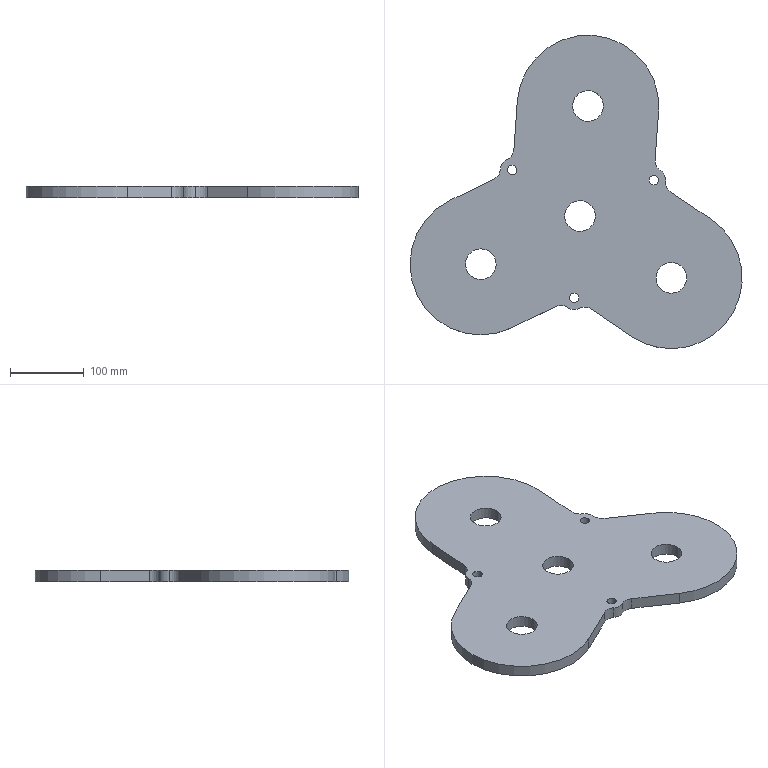Part | SolidWorks | features BaseBody 1 | 1 solid | 37 faces | box 450.446 x 425.125 x 16 mm | volume 1740357 mm3 | cylinder 29 | plane 8 | commonest cylinder face diameters 32 x11 41.6 x8 12.8 x6 192 x4
STEP:
#1=CARTESIAN_POINT('',(-327.08,104.201,479.4));
#2=VERTEX_POINT('',#1);
#3=CARTESIAN_POINT('',(-327.068,104.358,479.4));
#4=VERTEX_POINT('',#3);
#5=CARTESIAN_POINT('',(-311.122,103.052,479.4));
#6=DIRECTION('',(0.,0.,-1.));
#7=DIRECTION('',(-0.9974,0.07181,0.));
#8=AXIS2_PLACEMENT_3D('',#5,#6,#7);
#9=CIRCLE('',#8,16.);
#10=EDGE_CURVE('',#2,#4,#9,.T.);
#11=ORIENTED_EDGE('',*,*,#10,.F.);
#12=CARTESIAN_POINT('',(-327.08,104.201,463.4));
#13=VERTEX_POINT('',#12);
#14=CARTESIAN_POINT('',(-327.08,104.201,524.655));
#15=DIRECTION('',(0.,0.,-1.));
#16=VECTOR('',#15,1000.);
#17=LINE('',#14,#16);
#18=EDGE_CURVE('',#2,#13,#17,.T.);
#19=ORIENTED_EDGE('',*,*,#18,.T.);
#20=CARTESIAN_POINT('',(-327.068,104.358,463.4));
#21=VERTEX_POINT('',#20);
#22=CARTESIAN_POINT('',(-311.122,103.052,463.4));
#23=DIRECTION('',(0.,0.,1.));
#24=DIRECTION('',(-0.9974,0.07181,0.));
#25=AXIS2_PLACEMENT_3D('',#22,#23,#24);
#26=CIRCLE('',#25,16.);
#27=EDGE_CURVE('',#21,#13,#26,.T.);
#28=ORIENTED_EDGE('',*,*,#27,.F.);
#29=CARTESIAN_POINT('',(-327.068,104.358,524.655));
#30=DIRECTION('',(0.,0.,-1.));
#31=VECTOR('',#30,1000.);
#32=LINE('',#29,#31);
#33=EDGE_CURVE('',#4,#21,#32,.T.);
#34=ORIENTED_EDGE('',*,*,#33,.F.);
#35=EDGE_LOOP('',(#11,#19,#28,#34));
#36=FACE_OUTER_BOUND('',#35,.T.);
#37=CARTESIAN_POINT('',(-311.122,103.052,524.655));
#38=DIRECTION('',(0.,0.,-1.));
#39=DIRECTION('',(-0.9974,0.07181,0.));
#40=AXIS2_PLACEMENT_3D('',#37,#38,#39);
#41=CYLINDRICAL_SURFACE('',#40,16.);
#42=ADVANCED_FACE('',(#36),#41,.F.);
#43=CARTESIAN_POINT('',(-541.45,119.952,479.4));
#44=VERTEX_POINT('',#43);
#45=CARTESIAN_POINT('',(-528.683,119.033,479.4));
#46=VERTEX_POINT('',#45);
#47=CARTESIAN_POINT('',(-535.066,119.493,479.4));
#48=DIRECTION('',(0.,0.,1.));
#49=DIRECTION('',(-0.9974,0.07181,0.));
#50=AXIS2_PLACEMENT_3D('',#47,#48,#49);
#51=CIRCLE('',#50,6.4);
#52=EDGE_CURVE('',#44,#46,#51,.T.);
#53=ORIENTED_EDGE('',*,*,#52,.T.);
#54=CARTESIAN_POINT('',(-528.683,119.033,463.4));
#55=VERTEX_POINT('',#54);
#56=CARTESIAN_POINT('',(-528.683,119.033,524.655));
#57=DIRECTION('',(0.,0.,-1.));
#58=VECTOR('',#57,1000.);
#59=LINE('',#56,#58);
#60=EDGE_CURVE('',#46,#55,#59,.T.);
#61=ORIENTED_EDGE('',*,*,#60,.T.);
#62=CARTESIAN_POINT('',(-541.45,119.952,463.4));
#63=VERTEX_POINT('',#62);
#64=CARTESIAN_POINT('',(-535.066,119.493,463.4));
#65=DIRECTION('',(0.,0.,-1.));
#66=DIRECTION('',(-0.9974,0.07181,0.));
#67=AXIS2_PLACEMENT_3D('',#64,#65,#66);
#68=CIRCLE('',#67,6.4);
#69=EDGE_CURVE('',#55,#63,#68,.T.);
#70=ORIENTED_EDGE('',*,*,#69,.T.);
#71=CARTESIAN_POINT('',(-541.45,119.952,524.655));
#72=DIRECTION('',(0.,0.,-1.));
#73=VECTOR('',#72,1000.);
#74=LINE('',#71,#73);
#75=EDGE_CURVE('',#44,#63,#74,.T.);
#76=ORIENTED_EDGE('',*,*,#75,.F.);
#77=EDGE_LOOP('',(#53,#61,#70,#76));
#78=FACE_OUTER_BOUND('',#77,.T.);
#79=CARTESIAN_POINT('',(-535.066,119.493,524.655));
#80=DIRECTION('',(0.,0.,-1.));
#81=DIRECTION('',(-0.9974,0.07181,0.));
#82=AXIS2_PLACEMENT_3D('',#79,#80,#81);
#83=CYLINDRICAL_SURFACE('',#82,6.4);
#84=ADVANCED_FACE('',(#78),#83,.F.);
#85=CARTESIAN_POINT('',(-551.025,120.642,479.4));
#86=VERTEX_POINT('',#85);
#87=CARTESIAN_POINT('',(-551.036,120.484,479.4));
#88=VERTEX_POINT('',#87);
#89=CARTESIAN_POINT('',(-535.066,119.493,479.4));
#90=DIRECTION('',(0.,0.,1.));
#91=DIRECTION('',(-0.9974,0.07181,0.));
#92=AXIS2_PLACEMENT_3D('',#89,#90,#91);
#93=CIRCLE('',#92,16.);
#94=EDGE_CURVE('',#86,#88,#93,.T.);
#95=ORIENTED_EDGE('',*,*,#94,.F.);
#96=CARTESIAN_POINT('',(-551.025,120.642,463.4));
#97=VERTEX_POINT('',#96);
#98=CARTESIAN_POINT('',(-551.025,120.642,524.655));
#99=DIRECTION('',(0.,0.,-1.));
#100=VECTOR('',#99,1000.);
#101=LINE('',#98,#100);
#102=EDGE_CURVE('',#86,#97,#101,.T.);
#103=ORIENTED_EDGE('',*,*,#102,.T.);
#104=CARTESIAN_POINT('',(-551.036,120.484,463.4));
#105=VERTEX_POINT('',#104);
#106=CARTESIAN_POINT('',(-535.066,119.493,463.4));
#107=DIRECTION('',(0.,0.,-1.));
#108=DIRECTION('',(-0.9974,0.07181,0.));
#109=AXIS2_PLACEMENT_3D('',#106,#107,#108);
#110=CIRCLE('',#109,16.);
#111=EDGE_CURVE('',#105,#97,#110,.T.);
#112=ORIENTED_EDGE('',*,*,#111,.F.);
#113=CARTESIAN_POINT('',(-551.036,120.484,524.655));
#114=DIRECTION('',(0.,0.,1.));
#115=VECTOR('',#114,1000.);
#116=LINE('',#113,#115);
#117=EDGE_CURVE('',#105,#88,#116,.T.);
#118=ORIENTED_EDGE('',*,*,#117,.T.);
#119=EDGE_LOOP('',(#95,#103,#112,#118));
#120=FACE_OUTER_BOUND('',#119,.T.);
#121=CARTESIAN_POINT('',(-535.066,119.493,524.655));
#122=DIRECTION('',(0.,0.,-1.));
#123=DIRECTION('',(-0.9974,0.07181,0.));
#124=AXIS2_PLACEMENT_3D('',#121,#122,#123);
#125=CYLINDRICAL_SURFACE('',#124,16.);
#126=ADVANCED_FACE('',(#120),#125,.T.);
#127=CARTESIAN_POINT('',(-349.398,106.125,479.4));
#128=VERTEX_POINT('',#127);
#129=CARTESIAN_POINT('',(-336.631,105.205,479.4));
#130=VERTEX_POINT('',#129);
#131=CARTESIAN_POINT('',(-343.015,105.665,479.4));
#132=DIRECTION('',(0.,0.,1.));
#133=DIRECTION('',(-0.9974,0.07181,0.));
#134=AXIS2_PLACEMENT_3D('',#131,#132,#133);
#135=CIRCLE('',#134,6.4);
#136=EDGE_CURVE('',#128,#130,#135,.T.);
#137=ORIENTED_EDGE('',*,*,#136,.T.);
#138=CARTESIAN_POINT('',(-336.631,105.205,463.4));
#139=VERTEX_POINT('',#138);
#140=CARTESIAN_POINT('',(-336.631,105.205,524.655));
#141=DIRECTION('',(0.,0.,-1.));
#142=VECTOR('',#141,1000.);
#143=LINE('',#140,#142);
#144=EDGE_CURVE('',#130,#139,#143,.T.);
#145=ORIENTED_EDGE('',*,*,#144,.T.);
#146=CARTESIAN_POINT('',(-349.398,106.125,463.4));
#147=VERTEX_POINT('',#146);
#148=CARTESIAN_POINT('',(-343.015,105.665,463.4));
#149=DIRECTION('',(0.,0.,-1.));
#150=DIRECTION('',(-0.9974,0.07181,0.));
#151=AXIS2_PLACEMENT_3D('',#148,#149,#150);
#152=CIRCLE('',#151,6.4);
#153=EDGE_CURVE('',#139,#147,#152,.T.);
#154=ORIENTED_EDGE('',*,*,#153,.T.);
#155=CARTESIAN_POINT('',(-349.398,106.125,524.655));
#156=DIRECTION('',(0.,0.,-1.));
#157=VECTOR('',#156,1000.);
#158=LINE('',#155,#157);
#159=EDGE_CURVE('',#128,#147,#158,.T.);
#160=ORIENTED_EDGE('',*,*,#159,.F.);
#161=EDGE_LOOP('',(#137,#145,#154,#160));
#162=FACE_OUTER_BOUND('',#161,.T.);
#163=CARTESIAN_POINT('',(-343.015,105.665,524.655));
#164=DIRECTION('',(0.,0.,-1.));
#165=DIRECTION('',(-0.9974,0.07181,0.));
#166=AXIS2_PLACEMENT_3D('',#163,#164,#165);
#167=CYLINDRICAL_SURFACE('',#166,6.4);
#168=ADVANCED_FACE('',(#162),#167,.F.);
#169=CARTESIAN_POINT('',(-457.399,-53.283,479.4));
#170=VERTEX_POINT('',#169);
#171=CARTESIAN_POINT('',(-444.632,-54.202,479.4));
#172=VERTEX_POINT('',#171);
#173=CARTESIAN_POINT('',(-451.016,-53.743,479.4));
#174=DIRECTION('',(0.,0.,1.));
#175=DIRECTION('',(-0.9974,0.07181,0.));
#176=AXIS2_PLACEMENT_3D('',#173,#174,#175);
#177=CIRCLE('',#176,6.4);
#178=EDGE_CURVE('',#170,#172,#177,.T.);
#179=ORIENTED_EDGE('',*,*,#178,.T.);
#180=CARTESIAN_POINT('',(-444.632,-54.202,463.4));
#181=VERTEX_POINT('',#180);
#182=CARTESIAN_POINT('',(-444.632,-54.202,524.655));
#183=DIRECTION('',(0.,0.,-1.));
#184=VECTOR('',#183,1000.);
#185=LINE('',#182,#184);
#186=EDGE_CURVE('',#172,#181,#185,.T.);
#187=ORIENTED_EDGE('',*,*,#186,.T.);
#188=CARTESIAN_POINT('',(-457.399,-53.283,463.4));
#189=VERTEX_POINT('',#188);
#190=CARTESIAN_POINT('',(-451.016,-53.743,463.4));
#191=DIRECTION('',(0.,0.,-1.));
#192=DIRECTION('',(-0.9974,0.07181,0.));
#193=AXIS2_PLACEMENT_3D('',#190,#191,#192);
#194=CIRCLE('',#193,6.4);
#195=EDGE_CURVE('',#181,#189,#194,.T.);
#196=ORIENTED_EDGE('',*,*,#195,.T.);
#197=CARTESIAN_POINT('',(-457.399,-53.283,524.655));
#198=DIRECTION('',(0.,0.,-1.));
#199=VECTOR('',#198,1000.);
#200=LINE('',#197,#199);
#201=EDGE_CURVE('',#170,#189,#200,.T.);
#202=ORIENTED_EDGE('',*,*,#201,.F.);
#203=EDGE_LOOP('',(#179,#187,#196,#202));
#204=FACE_OUTER_BOUND('',#203,.T.);
#205=CARTESIAN_POINT('',(-451.016,-53.743,524.655));
#206=DIRECTION('',(0.,0.,-1.));
#207=DIRECTION('',(-0.9974,0.07181,0.));
#208=AXIS2_PLACEMENT_3D('',#205,#206,#207);
#209=CYLINDRICAL_SURFACE('',#208,6.4);
#210=ADVANCED_FACE('',(#204),#209,.F.);
#211=CARTESIAN_POINT('',(-556.881,-9.658,479.4));
#212=VERTEX_POINT('',#211);
#213=CARTESIAN_POINT('',(-598.373,-6.671,479.4));
#214=VERTEX_POINT('',#213);
#215=CARTESIAN_POINT('',(-577.627,-8.164,479.4));
#216=DIRECTION('',(0.,0.,-1.));
#217=DIRECTION('',(-0.9974,0.07181,0.));
#218=AXIS2_PLACEMENT_3D('',#215,#216,#217);
#219=CIRCLE('',#218,20.8);
#220=EDGE_CURVE('',#212,#214,#219,.T.);
#221=ORIENTED_EDGE('',*,*,#220,.F.);
#222=CARTESIAN_POINT('',(-556.881,-9.658,463.4));
#223=VERTEX_POINT('',#222);
#224=CARTESIAN_POINT('',(-556.881,-9.658,479.4));
#225=DIRECTION('',(0.,0.,-1.));
#226=VECTOR('',#225,1000.);
#227=LINE('',#224,#226);
#228=EDGE_CURVE('',#212,#223,#227,.T.);
#229=ORIENTED_EDGE('',*,*,#228,.T.);
#230=CARTESIAN_POINT('',(-598.373,-6.671,463.4));
#231=VERTEX_POINT('',#230);
#232=CARTESIAN_POINT('',(-577.627,-8.164,463.4));
#233=DIRECTION('',(0.,0.,-1.));
#234=DIRECTION('',(-0.9974,0.07181,0.));
#235=AXIS2_PLACEMENT_3D('',#232,#233,#234);
#236=CIRCLE('',#235,20.8);
#237=EDGE_CURVE('',#223,#231,#236,.T.);
#238=ORIENTED_EDGE('',*,*,#237,.T.);
#239=CARTESIAN_POINT('',(-598.373,-6.671,479.4));
#240=DIRECTION('',(0.,0.,-1.));
#241=VECTOR('',#240,1000.);
#242=LINE('',#239,#241);
#243=EDGE_CURVE('',#214,#231,#242,.T.);
#244=ORIENTED_EDGE('',*,*,#243,.F.);
#245=EDGE_LOOP('',(#221,#229,#238,#244));
#246=FACE_OUTER_BOUND('',#245,.T.);
#247=CARTESIAN_POINT('',(-577.627,-8.164,479.4));
#248=DIRECTION('',(0.,0.,-1.));
#249=DIRECTION('',(-0.9974,0.07181,0.));
#250=AXIS2_PLACEMENT_3D('',#247,#248,#249);
#251=CYLINDRICAL_SURFACE('',#250,20.8);
#252=ADVANCED_FACE('',(#246),#251,.F.);
#253=CARTESIAN_POINT('',(-298.435,-28.266,479.4));
#254=VERTEX_POINT('',#253);
#255=CARTESIAN_POINT('',(-339.927,-25.279,479.4));
#256=VERTEX_POINT('',#255);
#257=CARTESIAN_POINT('',(-319.181,-26.773,479.4));
#258=DIRECTION('',(0.,0.,-1.));
#259=DIRECTION('',(-0.9974,0.07181,0.));
#260=AXIS2_PLACEMENT_3D('',#257,#258,#259);
#261=CIRCLE('',#260,20.8);
#262=EDGE_CURVE('',#254,#256,#261,.T.);
#263=ORIENTED_EDGE('',*,*,#262,.F.);
#264=CARTESIAN_POINT('',(-298.435,-28.266,463.4));
#265=VERTEX_POINT('',#264);
#266=CARTESIAN_POINT('',(-298.435,-28.266,479.4));
#267=DIRECTION('',(0.,0.,-1.));
#268=VECTOR('',#267,1000.);
#269=LINE('',#266,#268);
#270=EDGE_CURVE('',#254,#265,#269,.T.);
#271=ORIENTED_EDGE('',*,*,#270,.T.);
#272=CARTESIAN_POINT('',(-339.927,-25.279,463.4));
#273=VERTEX_POINT('',#272);
#274=CARTESIAN_POINT('',(-319.181,-26.773,463.4));
#275=DIRECTION('',(0.,0.,-1.));
#276=DIRECTION('',(-0.9974,0.07181,0.));
#277=AXIS2_PLACEMENT_3D('',#274,#275,#276);
#278=CIRCLE('',#277,20.8);
#279=EDGE_CURVE('',#265,#273,#278,.T.);
#280=ORIENTED_EDGE('',*,*,#279,.T.);
#281=CARTESIAN_POINT('',(-339.927,-25.279,479.4));
#282=DIRECTION('',(0.,0.,-1.));
#283=VECTOR('',#282,1000.);
#284=LINE('',#281,#283);
#285=EDGE_CURVE('',#256,#273,#284,.T.);
#286=ORIENTED_EDGE('',*,*,#285,.F.);
#287=EDGE_LOOP('',(#263,#271,#280,#286));
#288=FACE_OUTER_BOUND('',#287,.T.);
#289=CARTESIAN_POINT('',(-319.181,-26.773,479.4));
#290=DIRECTION('',(0.,0.,-1.));
#291=DIRECTION('',(-0.9974,0.07181,0.));
#292=AXIS2_PLACEMENT_3D('',#289,#290,#291);
#293=CYLINDRICAL_SURFACE('',#292,20.8);
#294=ADVANCED_FACE('',(#288),#293,.F.);
#295=CARTESIAN_POINT('',(-422.286,55.645,479.4));
#296=VERTEX_POINT('',#295);
#297=CARTESIAN_POINT('',(-463.779,58.632,479.4));
#298=VERTEX_POINT('',#297);
#299=CARTESIAN_POINT('',(-443.032,57.138,479.4));
#300=DIRECTION('',(0.,0.,-1.));
#301=DIRECTION('',(-0.9974,0.07181,0.));
#302=AXIS2_PLACEMENT_3D('',#299,#300,#301);
#303=CIRCLE('',#302,20.8);
#304=EDGE_CURVE('',#296,#298,#303,.T.);
#305=ORIENTED_EDGE('',*,*,#304,.F.);
#306=CARTESIAN_POINT('',(-422.286,55.645,463.4));
#307=VERTEX_POINT('',#306);
#308=CARTESIAN_POINT('',(-422.286,55.645,479.4));
#309=DIRECTION('',(0.,0.,-1.));
#310=VECTOR('',#309,1000.);
#311=LINE('',#308,#310);
#312=EDGE_CURVE('',#296,#307,#311,.T.);
#313=ORIENTED_EDGE('',*,*,#312,.T.);
#314=CARTESIAN_POINT('',(-463.779,58.632,463.4));
#315=VERTEX_POINT('',#314);
#316=CARTESIAN_POINT('',(-443.032,57.138,463.4));
#317=DIRECTION('',(0.,0.,-1.));
#318=DIRECTION('',(-0.9974,0.07181,0.));
#319=AXIS2_PLACEMENT_3D('',#316,#317,#318);
#320=CIRCLE('',#319,20.8);
#321=EDGE_CURVE('',#307,#315,#320,.T.);
#322=ORIENTED_EDGE('',*,*,#321,.T.);
#323=CARTESIAN_POINT('',(-463.779,58.632,479.4));
#324=DIRECTION('',(0.,0.,-1.));
#325=VECTOR('',#324,1000.);
#326=LINE('',#323,#325);
#327=EDGE_CURVE('',#298,#315,#326,.T.);
#328=ORIENTED_EDGE('',*,*,#327,.F.);
#329=EDGE_LOOP('',(#305,#313,#322,#328));
#330=FACE_OUTER_BOUND('',#329,.T.);
#331=CARTESIAN_POINT('',(-443.032,57.138,479.4));
#332=DIRECTION('',(0.,0.,-1.));
#333=DIRECTION('',(-0.9974,0.07181,0.));
#334=AXIS2_PLACEMENT_3D('',#331,#332,#333);
#335=CYLINDRICAL_SURFACE('',#334,20.8);
#336=ADVANCED_FACE('',(#330),#335,.F.);
#337=CARTESIAN_POINT('',(-411.543,204.858,479.4));
#338=VERTEX_POINT('',#337);
#339=CARTESIAN_POINT('',(-453.035,207.846,479.4));
#340=VERTEX_POINT('',#339);
#341=CARTESIAN_POINT('',(-432.289,206.352,479.4));
#342=DIRECTION('',(0.,0.,-1.));
#343=DIRECTION('',(-0.9974,0.07181,0.));
#344=AXIS2_PLACEMENT_3D('',#341,#342,#343);
#345=CIRCLE('',#344,20.8);
#346=EDGE_CURVE('',#338,#340,#345,.T.);
#347=ORIENTED_EDGE('',*,*,#346,.F.);
#348=CARTESIAN_POINT('',(-411.543,204.858,463.4));
#349=VERTEX_POINT('',#348);
#350=CARTESIAN_POINT('',(-411.543,204.858,479.4));
#351=DIRECTION('',(0.,0.,-1.));
#352=VECTOR('',#351,1000.);
#353=LINE('',#350,#352);
#354=EDGE_CURVE('',#338,#349,#353,.T.);
#355=ORIENTED_EDGE('',*,*,#354,.T.);
#356=CARTESIAN_POINT('',(-453.035,207.846,463.4));
#357=VERTEX_POINT('',#356);
#358=CARTESIAN_POINT('',(-432.289,206.352,463.4));
#359=DIRECTION('',(0.,0.,-1.));
#360=DIRECTION('',(-0.9974,0.07181,0.));
#361=AXIS2_PLACEMENT_3D('',#358,#359,#360);
#362=CIRCLE('',#361,20.8);
#363=EDGE_CURVE('',#349,#357,#362,.T.);
#364=ORIENTED_EDGE('',*,*,#363,.T.);
#365=CARTESIAN_POINT('',(-453.035,207.846,479.4));
#366=DIRECTION('',(0.,0.,-1.));
#367=VECTOR('',#366,1000.);
#368=LINE('',#365,#367);
#369=EDGE_CURVE('',#340,#357,#368,.T.);
#370=ORIENTED_EDGE('',*,*,#369,.F.);
#371=EDGE_LOOP('',(#347,#355,#364,#370));
#372=FACE_OUTER_BOUND('',#371,.T.);
#373=CARTESIAN_POINT('',(-432.289,206.352,479.4));
#374=DIRECTION('',(0.,0.,-1.));
#375=DIRECTION('',(-0.9974,0.07181,0.));
#376=AXIS2_PLACEMENT_3D('',#373,#374,#375);
#377=CYLINDRICAL_SURFACE('',#376,20.8);
#378=ADVANCED_FACE('',(#372),#377,.F.);
#379=CARTESIAN_POINT('',(-223.429,-33.667,463.4));
#380=VERTEX_POINT('',#379);
#381=CARTESIAN_POINT('',(-373.028,-106.249,463.4));
#382=VERTEX_POINT('',#381);
#383=CARTESIAN_POINT('',(-319.181,-26.773,463.4));
#384=DIRECTION('',(0.,0.,-1.));
#385=DIRECTION('',(-0.9974,0.07181,0.));
#386=AXIS2_PLACEMENT_3D('',#383,#384,#385);
#387=CIRCLE('',#386,96.);
#388=EDGE_CURVE('',#380,#382,#387,.T.);
#389=ORIENTED_EDGE('',*,*,#388,.F.);
#390=CARTESIAN_POINT('',(-223.429,-33.667,479.4));
#391=VERTEX_POINT('',#390);
#392=CARTESIAN_POINT('',(-223.429,-33.667,463.4));
#393=DIRECTION('',(0.,0.,1.));
#394=VECTOR('',#393,1000.);
#395=LINE('',#392,#394);
#396=EDGE_CURVE('',#380,#391,#395,.T.);
#397=ORIENTED_EDGE('',*,*,#396,.T.);
#398=CARTESIAN_POINT('',(-373.028,-106.249,479.4));
#399=VERTEX_POINT('',#398);
#400=CARTESIAN_POINT('',(-319.181,-26.773,479.4));
#401=DIRECTION('',(0.,0.,-1.));
#402=DIRECTION('',(-0.9974,0.07181,0.));
#403=AXIS2_PLACEMENT_3D('',#400,#401,#402);
#404=CIRCLE('',#403,96.);
#405=EDGE_CURVE('',#391,#399,#404,.T.);
#406=ORIENTED_EDGE('',*,*,#405,.T.);
#407=CARTESIAN_POINT('',(-373.028,-106.249,463.4));
#408=DIRECTION('',(0.,0.,1.));
#409=VECTOR('',#408,1000.);
#410=LINE('',#407,#409);
#411=EDGE_CURVE('',#382,#399,#410,.T.);
#412=ORIENTED_EDGE('',*,*,#411,.F.);
#413=EDGE_LOOP('',(#389,#397,#406,#412));
#414=FACE_OUTER_BOUND('',#413,.T.);
#415=CARTESIAN_POINT('',(-319.181,-26.773,463.4));
#416=DIRECTION('',(0.,0.,1.));
#417=DIRECTION('',(0.9974,-0.07181,0.));
#418=AXIS2_PLACEMENT_3D('',#415,#416,#417);
#419=CYLINDRICAL_SURFACE('',#418,96.);
#420=ADVANCED_FACE('',(#414),#419,.T.);
#421=CARTESIAN_POINT('',(-532.791,147.27,463.4));
#422=VERTEX_POINT('',#421);
#423=CARTESIAN_POINT('',(-528.041,213.246,463.4));
#424=VERTEX_POINT('',#423);
#425=CARTESIAN_POINT('',(-533.477,137.743,463.4));
#426=DIRECTION('',(0.07181,0.9974,0.));
#427=VECTOR('',#426,1000.);
#428=LINE('',#425,#427);
#429=EDGE_CURVE('',#422,#424,#428,.T.);
#430=ORIENTED_EDGE('',*,*,#429,.F.);
#431=CARTESIAN_POINT('',(-532.791,147.27,479.4));
#432=VERTEX_POINT('',#431);
#433=CARTESIAN_POINT('',(-532.791,147.27,463.4));
#434=DIRECTION('',(0.,0.,1.));
#435=VECTOR('',#434,1000.);
#436=LINE('',#433,#435);
#437=EDGE_CURVE('',#422,#432,#436,.T.);
#438=ORIENTED_EDGE('',*,*,#437,.T.);
#439=CARTESIAN_POINT('',(-528.041,213.246,479.4));
#440=VERTEX_POINT('',#439);
#441=CARTESIAN_POINT('',(-533.477,137.743,479.4));
#442=DIRECTION('',(0.07181,0.9974,0.));
#443=VECTOR('',#442,1000.);
#444=LINE('',#441,#443);
#445=EDGE_CURVE('',#432,#440,#444,.T.);
#446=ORIENTED_EDGE('',*,*,#445,.T.);
#447=CARTESIAN_POINT('',(-528.041,213.246,463.4));
#448=DIRECTION('',(0.,0.,1.));
#449=VECTOR('',#448,1000.);
#450=LINE('',#447,#449);
#451=EDGE_CURVE('',#424,#440,#450,.T.);
#452=ORIENTED_EDGE('',*,*,#451,.F.);
#453=EDGE_LOOP('',(#430,#438,#446,#452));
#454=FACE_OUTER_BOUND('',#453,.T.);
#455=CARTESIAN_POINT('',(-533.477,137.743,463.4));
#456=DIRECTION('',(0.9974,-0.07181,0.));
#457=DIRECTION('',(-0.07181,-0.9974,0.));
#458=AXIS2_PLACEMENT_3D('',#455,#456,#457);
#459=PLANE('',#458);
#460=ADVANCED_FACE('',(#454),#459,.F.);
#461=CARTESIAN_POINT('',(-336.537,199.458,479.4));
#462=VERTEX_POINT('',#461);
#463=CARTESIAN_POINT('',(-432.289,206.352,479.4));
#464=DIRECTION('',(0.,0.,-1.));
#465=DIRECTION('',(-0.9974,0.07181,0.));
#466=AXIS2_PLACEMENT_3D('',#463,#464,#465);
#467=CIRCLE('',#466,96.);
#468=EDGE_CURVE('',#440,#462,#467,.T.);
#469=ORIENTED_EDGE('',*,*,#468,.T.);
#470=CARTESIAN_POINT('',(-336.537,199.458,463.4));
#471=VERTEX_POINT('',#470);
#472=CARTESIAN_POINT('',(-336.537,199.458,463.4));
#473=DIRECTION('',(0.,0.,1.));
#474=VECTOR('',#473,1000.);
#475=LINE('',#472,#474);
#476=EDGE_CURVE('',#471,#462,#475,.T.);
#477=ORIENTED_EDGE('',*,*,#476,.F.);
#478=CARTESIAN_POINT('',(-432.289,206.352,463.4));
#479=DIRECTION('',(0.,0.,-1.));
#480=DIRECTION('',(-0.9974,0.07181,0.));
#481=AXIS2_PLACEMENT_3D('',#478,#479,#480);
#482=CIRCLE('',#481,96.);
#483=EDGE_CURVE('',#424,#471,#482,.T.);
#484=ORIENTED_EDGE('',*,*,#483,.F.);
#485=ORIENTED_EDGE('',*,*,#451,.T.);
#486=EDGE_LOOP('',(#469,#477,#484,#485));
#487=FACE_OUTER_BOUND('',#486,.T.);
#488=CARTESIAN_POINT('',(-432.289,206.352,463.4));
#489=DIRECTION('',(0.,0.,1.));
#490=DIRECTION('',(0.9974,-0.07181,0.));
#491=AXIS2_PLACEMENT_3D('',#488,#489,#490);
#492=CYLINDRICAL_SURFACE('',#491,96.);
#493=ADVANCED_FACE('',(#487),#492,.T.);
#494=CARTESIAN_POINT('',(-341.287,133.482,479.4));
#495=VERTEX_POINT('',#494);
#496=CARTESIAN_POINT('',(-336.537,199.458,479.4));
#497=DIRECTION('',(-0.07181,-0.9974,0.));
#498=VECTOR('',#497,1000.);
#499=LINE('',#496,#498);
#500=EDGE_CURVE('',#462,#495,#499,.T.);
#501=ORIENTED_EDGE('',*,*,#500,.T.);
#502=CARTESIAN_POINT('',(-341.287,133.482,463.4));
#503=VERTEX_POINT('',#502);
#504=CARTESIAN_POINT('',(-341.287,133.482,463.4));
#505=DIRECTION('',(0.,0.,-1.));
#506=VECTOR('',#505,1000.);
#507=LINE('',#504,#506);
#508=EDGE_CURVE('',#495,#503,#507,.T.);
#509=ORIENTED_EDGE('',*,*,#508,.T.);
#510=CARTESIAN_POINT('',(-336.537,199.458,463.4));
#511=DIRECTION('',(-0.07181,-0.9974,0.));
#512=VECTOR('',#511,1000.);
#513=LINE('',#510,#512);
#514=EDGE_CURVE('',#471,#503,#513,.T.);
#515=ORIENTED_EDGE('',*,*,#514,.F.);
#516=ORIENTED_EDGE('',*,*,#476,.T.);
#517=EDGE_LOOP('',(#501,#509,#515,#516));
#518=FACE_OUTER_BOUND('',#517,.T.);
#519=CARTESIAN_POINT('',(-336.537,199.458,463.4));
#520=DIRECTION('',(-0.9974,0.07181,0.));
#521=DIRECTION('',(0.07181,0.9974,0.));
#522=AXIS2_PLACEMENT_3D('',#519,#520,#521);
#523=PLANE('',#522);
#524=ADVANCED_FACE('',(#518),#523,.F.);
#525=CARTESIAN_POINT('',(-320.096,89.806,463.4));
#526=VERTEX_POINT('',#525);
#527=CARTESIAN_POINT('',(-265.334,52.704,463.4));
#528=VERTEX_POINT('',#527);
#529=CARTESIAN_POINT('',(-328.004,95.164,463.4));
#530=DIRECTION('',(0.8279,-0.5609,0.));
#531=VECTOR('',#530,1000.);
#532=LINE('',#529,#531);
#533=EDGE_CURVE('',#526,#528,#532,.T.);
#534=ORIENTED_EDGE('',*,*,#533,.F.);
#535=CARTESIAN_POINT('',(-320.096,89.806,479.4));
#536=VERTEX_POINT('',#535);
#537=CARTESIAN_POINT('',(-320.096,89.806,463.4));
#538=DIRECTION('',(0.,0.,1.));
#539=VECTOR('',#538,1000.);
#540=LINE('',#537,#539);
#541=EDGE_CURVE('',#526,#536,#540,.T.);
#542=ORIENTED_EDGE('',*,*,#541,.T.);
#543=CARTESIAN_POINT('',(-265.334,52.704,479.4));
#544=VERTEX_POINT('',#543);
#545=CARTESIAN_POINT('',(-328.004,95.164,479.4));
#546=DIRECTION('',(0.8279,-0.5609,0.));
#547=VECTOR('',#546,1000.);
#548=LINE('',#545,#547);
#549=EDGE_CURVE('',#536,#544,#548,.T.);
#550=ORIENTED_EDGE('',*,*,#549,.T.);
#551=CARTESIAN_POINT('',(-265.334,52.704,463.4));
#552=DIRECTION('',(0.,0.,1.));
#553=VECTOR('',#552,1000.);
#554=LINE('',#551,#553);
#555=EDGE_CURVE('',#528,#544,#554,.T.);
#556=ORIENTED_EDGE('',*,*,#555,.F.);
#557=EDGE_LOOP('',(#534,#542,#550,#556));
#558=FACE_OUTER_BOUND('',#557,.T.);
#559=CARTESIAN_POINT('',(-328.004,95.164,463.4));
#560=DIRECTION('',(-0.5609,-0.8279,0.));
#561=DIRECTION('',(-0.8279,0.5609,0.));
#562=AXIS2_PLACEMENT_3D('',#559,#560,#561);
#563=PLANE('',#562);
#564=ADVANCED_FACE('',(#558),#563,.F.);
#565=ORIENTED_EDGE('',*,*,#396,.F.);
#566=CARTESIAN_POINT('',(-319.181,-26.773,463.4));
#567=DIRECTION('',(0.,0.,-1.));
#568=DIRECTION('',(-0.9974,0.07181,0.));
#569=AXIS2_PLACEMENT_3D('',#566,#567,#568);
#570=CIRCLE('',#569,96.);
#571=EDGE_CURVE('',#528,#380,#570,.T.);
#572=ORIENTED_EDGE('',*,*,#571,.F.);
#573=ORIENTED_EDGE('',*,*,#555,.T.);
#574=CARTESIAN_POINT('',(-319.181,-26.773,479.4));
#575=DIRECTION('',(0.,0.,-1.));
#576=DIRECTION('',(-0.9974,0.07181,0.));
#577=AXIS2_PLACEMENT_3D('',#574,#575,#576);
#578=CIRCLE('',#577,96.);
#579=EDGE_CURVE('',#544,#391,#578,.T.);
#580=ORIENTED_EDGE('',*,*,#579,.T.);
#581=EDGE_LOOP('',(#565,#572,#573,#580));
#582=FACE_OUTER_BOUND('',#581,.T.);
#583=CARTESIAN_POINT('',(-319.181,-26.773,463.4));
#584=DIRECTION('',(0.,0.,1.));
#585=DIRECTION('',(0.9974,-0.07181,0.));
#586=AXIS2_PLACEMENT_3D('',#583,#584,#585);
#587=CYLINDRICAL_SURFACE('',#586,96.);
#588=ADVANCED_FACE('',(#582),#587,.T.);
#589=CARTESIAN_POINT('',(-427.789,-69.148,479.4));
#590=VERTEX_POINT('',#589);
#591=CARTESIAN_POINT('',(-373.028,-106.249,479.4));
#592=DIRECTION('',(-0.8279,0.5609,0.));
#593=VECTOR('',#592,1000.);
#594=LINE('',#591,#593);
#595=EDGE_CURVE('',#399,#590,#594,.T.);
#596=ORIENTED_EDGE('',*,*,#595,.T.);
#597=CARTESIAN_POINT('',(-427.789,-69.148,463.4));
#598=VERTEX_POINT('',#597);
#599=CARTESIAN_POINT('',(-427.789,-69.148,463.4));
#600=DIRECTION('',(0.,0.,-1.));
#601=VECTOR('',#600,1000.);
#602=LINE('',#599,#601);
#603=EDGE_CURVE('',#590,#598,#602,.T.);
#604=ORIENTED_EDGE('',*,*,#603,.T.);
#605=CARTESIAN_POINT('',(-373.028,-106.249,463.4));
#606=DIRECTION('',(-0.8279,0.5609,0.));
#607=VECTOR('',#606,1000.);
#608=LINE('',#605,#607);
#609=EDGE_CURVE('',#382,#598,#608,.T.);
#610=ORIENTED_EDGE('',*,*,#609,.F.);
#611=ORIENTED_EDGE('',*,*,#411,.T.);
#612=EDGE_LOOP('',(#596,#604,#610,#611));
#613=FACE_OUTER_BOUND('',#612,.T.);
#614=CARTESIAN_POINT('',(-373.028,-106.249,463.4));
#615=DIRECTION('',(0.5609,0.8279,0.));
#616=DIRECTION('',(0.8279,-0.5609,0.));
#617=AXIS2_PLACEMENT_3D('',#614,#615,#616);
#618=PLANE('',#617);
#619=ADVANCED_FACE('',(#613),#618,.F.);
#620=CARTESIAN_POINT('',(-476.209,-65.661,463.4));
#621=VERTEX_POINT('',#620);
#622=CARTESIAN_POINT('',(-535.721,-94.535,463.4));
#623=VERTEX_POINT('',#622);
#624=CARTESIAN_POINT('',(-467.615,-61.491,463.4));
#625=DIRECTION('',(-0.8997,-0.4365,0.));
#626=VECTOR('',#625,1000.);
#627=LINE('',#624,#626);
#628=EDGE_CURVE('',#621,#623,#627,.T.);
#629=ORIENTED_EDGE('',*,*,#628,.F.);
#630=CARTESIAN_POINT('',(-476.209,-65.661,479.4));
#631=VERTEX_POINT('',#630);
#632=CARTESIAN_POINT('',(-476.209,-65.661,463.4));
#633=DIRECTION('',(0.,0.,1.));
#634=VECTOR('',#633,1000.);
#635=LINE('',#632,#634);
#636=EDGE_CURVE('',#621,#631,#635,.T.);
#637=ORIENTED_EDGE('',*,*,#636,.T.);
#638=CARTESIAN_POINT('',(-535.721,-94.535,479.4));
#639=VERTEX_POINT('',#638);
#640=CARTESIAN_POINT('',(-467.615,-61.491,479.4));
#641=DIRECTION('',(-0.8997,-0.4365,0.));
#642=VECTOR('',#641,1000.);
#643=LINE('',#640,#642);
#644=EDGE_CURVE('',#631,#639,#643,.T.);
#645=ORIENTED_EDGE('',*,*,#644,.T.);
#646=CARTESIAN_POINT('',(-535.721,-94.535,463.4));
#647=DIRECTION('',(0.,0.,1.));
#648=VECTOR('',#647,1000.);
#649=LINE('',#646,#648);
#650=EDGE_CURVE('',#623,#639,#649,.T.);
#651=ORIENTED_EDGE('',*,*,#650,.F.);
#652=EDGE_LOOP('',(#629,#637,#645,#651));
#653=FACE_OUTER_BOUND('',#652,.T.);
#654=CARTESIAN_POINT('',(-467.615,-61.491,463.4));
#655=DIRECTION('',(-0.4365,0.8997,0.));
#656=DIRECTION('',(0.8997,0.4365,0.));
#657=AXIS2_PLACEMENT_3D('',#654,#655,#656);
#658=PLANE('',#657);
#659=ADVANCED_FACE('',(#653),#658,.F.);
#660=CARTESIAN_POINT('',(-619.532,78.206,479.4));
#661=VERTEX_POINT('',#660);
#662=CARTESIAN_POINT('',(-577.627,-8.164,479.4));
#663=DIRECTION('',(0.,0.,-1.));
#664=DIRECTION('',(-0.9974,0.07181,0.));
#665=AXIS2_PLACEMENT_3D('',#662,#663,#664);
#666=CIRCLE('',#665,96.);
#667=EDGE_CURVE('',#639,#661,#666,.T.);
#668=ORIENTED_EDGE('',*,*,#667,.T.);
#669=CARTESIAN_POINT('',(-619.532,78.206,463.4));
#670=VERTEX_POINT('',#669);
#671=CARTESIAN_POINT('',(-619.532,78.206,463.4));
#672=DIRECTION('',(0.,0.,1.));
#673=VECTOR('',#672,1000.);
#674=LINE('',#671,#673);
#675=EDGE_CURVE('',#670,#661,#674,.T.);
#676=ORIENTED_EDGE('',*,*,#675,.F.);
#677=CARTESIAN_POINT('',(-577.627,-8.164,463.4));
#678=DIRECTION('',(0.,0.,-1.));
#679=DIRECTION('',(-0.9974,0.07181,0.));
#680=AXIS2_PLACEMENT_3D('',#677,#678,#679);
#681=CIRCLE('',#680,96.);
#682=EDGE_CURVE('',#623,#670,#681,.T.);
#683=ORIENTED_EDGE('',*,*,#682,.F.);
#684=ORIENTED_EDGE('',*,*,#650,.T.);
#685=EDGE_LOOP('',(#668,#676,#683,#684));
#686=FACE_OUTER_BOUND('',#685,.T.);
#687=CARTESIAN_POINT('',(-577.627,-8.164,463.4));
#688=DIRECTION('',(0.,0.,1.));
#689=DIRECTION('',(0.9974,-0.07181,0.));
#690=AXIS2_PLACEMENT_3D('',#687,#688,#689);
#691=CYLINDRICAL_SURFACE('',#690,96.);
#692=ADVANCED_FACE('',(#686),#691,.T.);
#693=CARTESIAN_POINT('',(-560.021,107.08,479.4));
#694=VERTEX_POINT('',#693);
#695=CARTESIAN_POINT('',(-619.532,78.206,479.4));
#696=DIRECTION('',(0.8997,0.4365,0.));
#697=VECTOR('',#696,1000.);
#698=LINE('',#695,#697);
#699=EDGE_CURVE('',#661,#694,#698,.T.);
#700=ORIENTED_EDGE('',*,*,#699,.T.);
#701=CARTESIAN_POINT('',(-560.021,107.08,463.4));
#702=VERTEX_POINT('',#701);
#703=CARTESIAN_POINT('',(-560.021,107.08,463.4));
#704=DIRECTION('',(0.,0.,-1.));
#705=VECTOR('',#704,1000.);
#706=LINE('',#703,#705);
#707=EDGE_CURVE('',#694,#702,#706,.T.);
#708=ORIENTED_EDGE('',*,*,#707,.T.);
#709=CARTESIAN_POINT('',(-619.532,78.206,463.4));
#710=DIRECTION('',(0.8997,0.4365,0.));
#711=VECTOR('',#710,1000.);
#712=LINE('',#709,#711);
#713=EDGE_CURVE('',#670,#702,#712,.T.);
#714=ORIENTED_EDGE('',*,*,#713,.F.);
#715=ORIENTED_EDGE('',*,*,#675,.T.);
#716=EDGE_LOOP('',(#700,#708,#714,#715));
#717=FACE_OUTER_BOUND('',#716,.T.);
#718=CARTESIAN_POINT('',(-619.532,78.206,463.4));
#719=DIRECTION('',(0.4365,-0.8997,0.));
#720=DIRECTION('',(-0.8997,-0.4365,0.));
#721=AXIS2_PLACEMENT_3D('',#718,#719,#720);
#722=PLANE('',#721);
#723=ADVANCED_FACE('',(#717),#722,.F.);
#724=CARTESIAN_POINT('',(-535.066,119.493,463.4));
#725=DIRECTION('',(0.,0.,-1.));
#726=DIRECTION('',(-0.9974,0.07181,0.));
#727=AXIS2_PLACEMENT_3D('',#724,#725,#726);
#728=CIRCLE('',#727,6.4);
#729=EDGE_CURVE('',#63,#55,#728,.T.);
#730=ORIENTED_EDGE('',*,*,#729,.F.);
#731=ORIENTED_EDGE('',*,*,#69,.F.);
#732=EDGE_LOOP('',(#730,#731));
#733=FACE_BOUND('',#732,.T.);
#734=CARTESIAN_POINT('',(-343.015,105.665,463.4));
#735=DIRECTION('',(0.,0.,-1.));
#736=DIRECTION('',(-0.9974,0.07181,0.));
#737=AXIS2_PLACEMENT_3D('',#734,#735,#736);
#738=CIRCLE('',#737,6.4);
#739=EDGE_CURVE('',#147,#139,#738,.T.);
#740=ORIENTED_EDGE('',*,*,#739,.F.);
#741=ORIENTED_EDGE('',*,*,#153,.F.);
#742=EDGE_LOOP('',(#740,#741));
#743=FACE_BOUND('',#742,.T.);
#744=CARTESIAN_POINT('',(-451.016,-53.743,463.4));
#745=DIRECTION('',(0.,0.,-1.));
#746=DIRECTION('',(-0.9974,0.07181,0.));
#747=AXIS2_PLACEMENT_3D('',#744,#745,#746);
#748=CIRCLE('',#747,6.4);
#749=EDGE_CURVE('',#189,#181,#748,.T.);
#750=ORIENTED_EDGE('',*,*,#749,.F.);
#751=ORIENTED_EDGE('',*,*,#195,.F.);
#752=EDGE_LOOP('',(#750,#751));
#753=FACE_BOUND('',#752,.T.);
#754=ORIENTED_EDGE('',*,*,#713,.T.);
#755=CARTESIAN_POINT('',(-567.005,121.476,463.4));
#756=DIRECTION('',(0.,0.,1.));
#757=DIRECTION('',(-0.9974,0.07181,0.));
#758=AXIS2_PLACEMENT_3D('',#755,#756,#757);
#759=CIRCLE('',#758,16.);
#760=EDGE_CURVE('',#702,#105,#759,.T.);
#761=ORIENTED_EDGE('',*,*,#760,.T.);
#762=ORIENTED_EDGE('',*,*,#111,.T.);
#763=CARTESIAN_POINT('',(-541.908,133.956,463.4));
#764=VERTEX_POINT('',#763);
#765=CARTESIAN_POINT('',(-535.066,119.493,463.4));
#766=DIRECTION('',(0.,0.,-1.));
#767=DIRECTION('',(-0.9974,0.07181,0.));
#768=AXIS2_PLACEMENT_3D('',#765,#766,#767);
#769=CIRCLE('',#768,16.);
#770=EDGE_CURVE('',#97,#764,#769,.T.);
#771=ORIENTED_EDGE('',*,*,#770,.T.);
#772=CARTESIAN_POINT('',(-548.75,148.419,463.4));
#773=DIRECTION('',(0.,0.,1.));
#774=DIRECTION('',(-0.9974,0.07181,0.));
#775=AXIS2_PLACEMENT_3D('',#772,#773,#774);
#776=CIRCLE('',#775,16.);
#777=EDGE_CURVE('',#764,#422,#776,.T.);
#778=ORIENTED_EDGE('',*,*,#777,.T.);
#779=ORIENTED_EDGE('',*,*,#429,.T.);
#780=ORIENTED_EDGE('',*,*,#483,.T.);
#781=ORIENTED_EDGE('',*,*,#514,.T.);
#782=CARTESIAN_POINT('',(-334.172,118.999,463.4));
#783=VERTEX_POINT('',#782);
#784=CARTESIAN_POINT('',(-325.328,132.333,463.4));
#785=DIRECTION('',(0.,0.,1.));
#786=DIRECTION('',(-0.9974,0.07181,0.));
#787=AXIS2_PLACEMENT_3D('',#784,#785,#786);
#788=CIRCLE('',#787,16.);
#789=EDGE_CURVE('',#503,#783,#788,.T.);
#790=ORIENTED_EDGE('',*,*,#789,.T.);
#791=CARTESIAN_POINT('',(-343.015,105.665,463.4));
#792=DIRECTION('',(0.,0.,-1.));
#793=DIRECTION('',(-0.9974,0.07181,0.));
#794=AXIS2_PLACEMENT_3D('',#791,#792,#793);
#795=CIRCLE('',#794,16.);
#796=EDGE_CURVE('',#783,#21,#795,.T.);
#797=ORIENTED_EDGE('',*,*,#796,.T.);
#798=ORIENTED_EDGE('',*,*,#27,.T.);
#799=CARTESIAN_POINT('',(-311.122,103.052,463.4));
#800=DIRECTION('',(0.,0.,1.));
#801=DIRECTION('',(-0.9974,0.07181,0.));
#802=AXIS2_PLACEMENT_3D('',#799,#800,#801);
#803=CIRCLE('',#802,16.);
#804=EDGE_CURVE('',#13,#526,#803,.T.);
#805=ORIENTED_EDGE('',*,*,#804,.T.);
#806=ORIENTED_EDGE('',*,*,#533,.T.);
#807=ORIENTED_EDGE('',*,*,#571,.T.);
#808=ORIENTED_EDGE('',*,*,#388,.T.);
#809=ORIENTED_EDGE('',*,*,#609,.T.);
#810=CARTESIAN_POINT('',(-443.89,-68.068,463.4));
#811=VERTEX_POINT('',#810);
#812=CARTESIAN_POINT('',(-436.764,-82.394,463.4));
#813=DIRECTION('',(0.,0.,1.));
#814=DIRECTION('',(-0.9974,0.07181,0.));
#815=AXIS2_PLACEMENT_3D('',#812,#813,#814);
#816=CIRCLE('',#815,16.);
#817=EDGE_CURVE('',#598,#811,#816,.T.);
#818=ORIENTED_EDGE('',*,*,#817,.T.);
#819=CARTESIAN_POINT('',(-460.12,-66.9,463.4));
#820=VERTEX_POINT('',#819);
#821=CARTESIAN_POINT('',(-451.016,-53.743,463.4));
#822=DIRECTION('',(0.,0.,-1.));
#823=DIRECTION('',(-0.9974,0.07181,0.));
#824=AXIS2_PLACEMENT_3D('',#821,#822,#823);
#825=CIRCLE('',#824,16.);
#826=EDGE_CURVE('',#811,#820,#825,.T.);
#827=ORIENTED_EDGE('',*,*,#826,.T.);
#828=CARTESIAN_POINT('',(-469.225,-80.056,463.4));
#829=DIRECTION('',(0.,0.,1.));
#830=DIRECTION('',(-0.9974,0.07181,0.));
#831=AXIS2_PLACEMENT_3D('',#828,#829,#830);
#832=CIRCLE('',#831,16.);
#833=EDGE_CURVE('',#820,#621,#832,.T.);
#834=ORIENTED_EDGE('',*,*,#833,.T.);
#835=ORIENTED_EDGE('',*,*,#628,.T.);
#836=ORIENTED_EDGE('',*,*,#682,.T.);
#837=EDGE_LOOP('',(#754,#761,#762,#771,#778,#779,#780,#781,#790,#797,#798,#805,#806,#807,#808,#809,#818,#827,#834,#835,#836));
#838=FACE_OUTER_BOUND('',#837,.T.);
#839=CARTESIAN_POINT('',(-577.627,-8.164,463.4));
#840=DIRECTION('',(0.,0.,-1.));
#841=DIRECTION('',(-0.9974,0.07181,0.));
#842=AXIS2_PLACEMENT_3D('',#839,#840,#841);
#843=CIRCLE('',#842,20.8);
#844=EDGE_CURVE('',#231,#223,#843,.T.);
#845=ORIENTED_EDGE('',*,*,#844,.F.);
#846=ORIENTED_EDGE('',*,*,#237,.F.);
#847=EDGE_LOOP('',(#845,#846));
#848=FACE_BOUND('',#847,.T.);
#849=CARTESIAN_POINT('',(-319.181,-26.773,463.4));
#850=DIRECTION('',(0.,0.,-1.));
#851=DIRECTION('',(-0.9974,0.07181,0.));
#852=AXIS2_PLACEMENT_3D('',#849,#850,#851);
#853=CIRCLE('',#852,20.8);
#854=EDGE_CURVE('',#273,#265,#853,.T.);
#855=ORIENTED_EDGE('',*,*,#854,.F.);
#856=ORIENTED_EDGE('',*,*,#279,.F.);
#857=EDGE_LOOP('',(#855,#856));
#858=FACE_BOUND('',#857,.T.);
#859=CARTESIAN_POINT('',(-443.032,57.138,463.4));
#860=DIRECTION('',(0.,0.,-1.));
#861=DIRECTION('',(-0.9974,0.07181,0.));
#862=AXIS2_PLACEMENT_3D('',#859,#860,#861);
#863=CIRCLE('',#862,20.8);
#864=EDGE_CURVE('',#315,#307,#863,.T.);
#865=ORIENTED_EDGE('',*,*,#864,.F.);
#866=ORIENTED_EDGE('',*,*,#321,.F.);
#867=EDGE_LOOP('',(#865,#866));
#868=FACE_BOUND('',#867,.T.);
#869=CARTESIAN_POINT('',(-432.289,206.352,463.4));
#870=DIRECTION('',(0.,0.,-1.));
#871=DIRECTION('',(-0.9974,0.07181,0.));
#872=AXIS2_PLACEMENT_3D('',#869,#870,#871);
#873=CIRCLE('',#872,20.8);
#874=EDGE_CURVE('',#357,#349,#873,.T.);
#875=ORIENTED_EDGE('',*,*,#874,.F.);
#876=ORIENTED_EDGE('',*,*,#363,.F.);
#877=EDGE_LOOP('',(#875,#876));
#878=FACE_BOUND('',#877,.T.);
#879=CARTESIAN_POINT('',(-432.289,206.352,463.4));
#880=DIRECTION('',(0.,0.,-1.));
#881=DIRECTION('',(-0.9974,0.07181,0.));
#882=AXIS2_PLACEMENT_3D('',#879,#880,#881);
#883=PLANE('',#882);
#884=ADVANCED_FACE('',(#733,#743,#753,#838,#848,#858,#868,#878),#883,.T.);
#885=ORIENTED_EDGE('',*,*,#52,.F.);
#886=CARTESIAN_POINT('',(-535.066,119.493,479.4));
#887=DIRECTION('',(0.,0.,1.));
#888=DIRECTION('',(-0.9974,0.07181,0.));
#889=AXIS2_PLACEMENT_3D('',#886,#887,#888);
#890=CIRCLE('',#889,6.4);
#891=EDGE_CURVE('',#46,#44,#890,.T.);
#892=ORIENTED_EDGE('',*,*,#891,.F.);
#893=EDGE_LOOP('',(#885,#892));
#894=FACE_BOUND('',#893,.T.);
#895=ORIENTED_EDGE('',*,*,#136,.F.);
#896=CARTESIAN_POINT('',(-343.015,105.665,479.4));
#897=DIRECTION('',(0.,0.,1.));
#898=DIRECTION('',(-0.9974,0.07181,0.));
#899=AXIS2_PLACEMENT_3D('',#896,#897,#898);
#900=CIRCLE('',#899,6.4);
#901=EDGE_CURVE('',#130,#128,#900,.T.);
#902=ORIENTED_EDGE('',*,*,#901,.F.);
#903=EDGE_LOOP('',(#895,#902));
#904=FACE_BOUND('',#903,.T.);
#905=ORIENTED_EDGE('',*,*,#178,.F.);
#906=CARTESIAN_POINT('',(-451.016,-53.743,479.4));
#907=DIRECTION('',(0.,0.,1.));
#908=DIRECTION('',(-0.9974,0.07181,0.));
#909=AXIS2_PLACEMENT_3D('',#906,#907,#908);
#910=CIRCLE('',#909,6.4);
#911=EDGE_CURVE('',#172,#170,#910,.T.);
#912=ORIENTED_EDGE('',*,*,#911,.F.);
#913=EDGE_LOOP('',(#905,#912));
#914=FACE_BOUND('',#913,.T.);
#915=CARTESIAN_POINT('',(-577.627,-8.164,479.4));
#916=DIRECTION('',(0.,0.,-1.));
#917=DIRECTION('',(-0.9974,0.07181,0.));
#918=AXIS2_PLACEMENT_3D('',#915,#916,#917);
#919=CIRCLE('',#918,20.8);
#920=EDGE_CURVE('',#214,#212,#919,.T.);
#921=ORIENTED_EDGE('',*,*,#920,.T.);
#922=ORIENTED_EDGE('',*,*,#220,.T.);
#923=EDGE_LOOP('',(#921,#922));
#924=FACE_BOUND('',#923,.T.);
#925=CARTESIAN_POINT('',(-319.181,-26.773,479.4));
#926=DIRECTION('',(0.,0.,-1.));
#927=DIRECTION('',(-0.9974,0.07181,0.));
#928=AXIS2_PLACEMENT_3D('',#925,#926,#927);
#929=CIRCLE('',#928,20.8);
#930=EDGE_CURVE('',#256,#254,#929,.T.);
#931=ORIENTED_EDGE('',*,*,#930,.T.);
#932=ORIENTED_EDGE('',*,*,#262,.T.);
#933=EDGE_LOOP('',(#931,#932));
#934=FACE_BOUND('',#933,.T.);
#935=CARTESIAN_POINT('',(-443.032,57.138,479.4));
#936=DIRECTION('',(0.,0.,-1.));
#937=DIRECTION('',(-0.9974,0.07181,0.));
#938=AXIS2_PLACEMENT_3D('',#935,#936,#937);
#939=CIRCLE('',#938,20.8);
#940=EDGE_CURVE('',#298,#296,#939,.T.);
#941=ORIENTED_EDGE('',*,*,#940,.T.);
#942=ORIENTED_EDGE('',*,*,#304,.T.);
#943=EDGE_LOOP('',(#941,#942));
#944=FACE_BOUND('',#943,.T.);
#945=CARTESIAN_POINT('',(-432.289,206.352,479.4));
#946=DIRECTION('',(0.,0.,-1.));
#947=DIRECTION('',(-0.9974,0.07181,0.));
#948=AXIS2_PLACEMENT_3D('',#945,#946,#947);
#949=CIRCLE('',#948,20.8);
#950=EDGE_CURVE('',#340,#338,#949,.T.);
#951=ORIENTED_EDGE('',*,*,#950,.T.);
#952=ORIENTED_EDGE('',*,*,#346,.T.);
#953=EDGE_LOOP('',(#951,#952));
#954=FACE_BOUND('',#953,.T.);
#955=ORIENTED_EDGE('',*,*,#445,.F.);
#956=CARTESIAN_POINT('',(-541.908,133.956,479.4));
#957=VERTEX_POINT('',#956);
#958=CARTESIAN_POINT('',(-548.75,148.419,479.4));
#959=DIRECTION('',(0.,0.,-1.));
#960=DIRECTION('',(-0.9974,0.07181,0.));
#961=AXIS2_PLACEMENT_3D('',#958,#959,#960);
#962=CIRCLE('',#961,16.);
#963=EDGE_CURVE('',#432,#957,#962,.T.);
#964=ORIENTED_EDGE('',*,*,#963,.T.);
#965=CARTESIAN_POINT('',(-535.066,119.493,479.4));
#966=DIRECTION('',(0.,0.,1.));
#967=DIRECTION('',(-0.9974,0.07181,0.));
#968=AXIS2_PLACEMENT_3D('',#965,#966,#967);
#969=CIRCLE('',#968,16.);
#970=EDGE_CURVE('',#957,#86,#969,.T.);
#971=ORIENTED_EDGE('',*,*,#970,.T.);
#972=ORIENTED_EDGE('',*,*,#94,.T.);
#973=CARTESIAN_POINT('',(-567.005,121.476,479.4));
#974=DIRECTION('',(0.,0.,-1.));
#975=DIRECTION('',(-0.9974,0.07181,0.));
#976=AXIS2_PLACEMENT_3D('',#973,#974,#975);
#977=CIRCLE('',#976,16.);
#978=EDGE_CURVE('',#88,#694,#977,.T.);
#979=ORIENTED_EDGE('',*,*,#978,.T.);
#980=ORIENTED_EDGE('',*,*,#699,.F.);
#981=ORIENTED_EDGE('',*,*,#667,.F.);
#982=ORIENTED_EDGE('',*,*,#644,.F.);
#983=CARTESIAN_POINT('',(-460.12,-66.9,479.4));
#984=VERTEX_POINT('',#983);
#985=CARTESIAN_POINT('',(-469.225,-80.056,479.4));
#986=DIRECTION('',(0.,0.,-1.));
#987=DIRECTION('',(-0.9974,0.07181,0.));
#988=AXIS2_PLACEMENT_3D('',#985,#986,#987);
#989=CIRCLE('',#988,16.);
#990=EDGE_CURVE('',#631,#984,#989,.T.);
#991=ORIENTED_EDGE('',*,*,#990,.T.);
#992=CARTESIAN_POINT('',(-443.89,-68.068,479.4));
#993=VERTEX_POINT('',#992);
#994=CARTESIAN_POINT('',(-451.016,-53.743,479.4));
#995=DIRECTION('',(0.,0.,1.));
#996=DIRECTION('',(-0.9974,0.07181,0.));
#997=AXIS2_PLACEMENT_3D('',#994,#995,#996);
#998=CIRCLE('',#997,16.);
#999=EDGE_CURVE('',#984,#993,#998,.T.);
#1000=ORIENTED_EDGE('',*,*,#999,.T.);
#1001=CARTESIAN_POINT('',(-436.764,-82.394,479.4));
#1002=DIRECTION('',(0.,0.,-1.));
#1003=DIRECTION('',(-0.9974,0.07181,0.));
#1004=AXIS2_PLACEMENT_3D('',#1001,#1002,#1003);
#1005=CIRCLE('',#1004,16.);
#1006=EDGE_CURVE('',#993,#590,#1005,.T.);
#1007=ORIENTED_EDGE('',*,*,#1006,.T.);
#1008=ORIENTED_EDGE('',*,*,#595,.F.);
#1009=ORIENTED_EDGE('',*,*,#405,.F.);
#1010=ORIENTED_EDGE('',*,*,#579,.F.);
#1011=ORIENTED_EDGE('',*,*,#549,.F.);
#1012=CARTESIAN_POINT('',(-311.122,103.052,479.4));
#1013=DIRECTION('',(0.,0.,-1.));
#1014=DIRECTION('',(-0.9974,0.07181,0.));
#1015=AXIS2_PLACEMENT_3D('',#1012,#1013,#1014);
#1016=CIRCLE('',#1015,16.);
#1017=EDGE_CURVE('',#536,#2,#1016,.T.);
#1018=ORIENTED_EDGE('',*,*,#1017,.T.);
#1019=ORIENTED_EDGE('',*,*,#10,.T.);
#1020=CARTESIAN_POINT('',(-334.172,118.999,479.4));
#1021=VERTEX_POINT('',#1020);
#1022=CARTESIAN_POINT('',(-343.015,105.665,479.4));
#1023=DIRECTION('',(0.,0.,1.));
#1024=DIRECTION('',(-0.9974,0.07181,0.));
#1025=AXIS2_PLACEMENT_3D('',#1022,#1023,#1024);
#1026=CIRCLE('',#1025,16.);
#1027=EDGE_CURVE('',#4,#1021,#1026,.T.);
#1028=ORIENTED_EDGE('',*,*,#1027,.T.);
#1029=CARTESIAN_POINT('',(-325.328,132.333,479.4));
#1030=DIRECTION('',(0.,0.,-1.));
#1031=DIRECTION('',(-0.9974,0.07181,0.));
#1032=AXIS2_PLACEMENT_3D('',#1029,#1030,#1031);
#1033=CIRCLE('',#1032,16.);
#1034=EDGE_CURVE('',#1021,#495,#1033,.T.);
#1035=ORIENTED_EDGE('',*,*,#1034,.T.);
#1036=ORIENTED_EDGE('',*,*,#500,.F.);
#1037=ORIENTED_EDGE('',*,*,#468,.F.);
#1038=EDGE_LOOP('',(#955,#964,#971,#972,#979,#980,#981,#982,#991,#1000,#1007,#1008,#1009,#1010,#1011,#1018,#1019,#1028,#1035,#1036,#1037));
#1039=FACE_OUTER_BOUND('',#1038,.T.);
#1040=CARTESIAN_POINT('',(-432.289,206.352,479.4));
#1041=DIRECTION('',(0.,0.,-1.));
#1042=DIRECTION('',(-0.9974,0.07181,0.));
#1043=AXIS2_PLACEMENT_3D('',#1040,#1041,#1042);
#1044=PLANE('',#1043);
#1045=ADVANCED_FACE('',(#894,#904,#914,#924,#934,#944,#954,#1039),#1044,.F.);
#1046=ORIENTED_EDGE('',*,*,#354,.F.);
#1047=ORIENTED_EDGE('',*,*,#950,.F.);
#1048=ORIENTED_EDGE('',*,*,#369,.T.);
#1049=ORIENTED_EDGE('',*,*,#874,.T.);
#1050=EDGE_LOOP('',(#1046,#1047,#1048,#1049));
#1051=FACE_OUTER_BOUND('',#1050,.T.);
#1052=CARTESIAN_POINT('',(-432.289,206.352,479.4));
#1053=DIRECTION('',(0.,0.,-1.));
#1054=DIRECTION('',(-0.9974,0.07181,0.));
#1055=AXIS2_PLACEMENT_3D('',#1052,#1053,#1054);
#1056=CYLINDRICAL_SURFACE('',#1055,20.8);
#1057=ADVANCED_FACE('',(#1051),#1056,.F.);
#1058=ORIENTED_EDGE('',*,*,#312,.F.);
#1059=ORIENTED_EDGE('',*,*,#940,.F.);
#1060=ORIENTED_EDGE('',*,*,#327,.T.);
#1061=ORIENTED_EDGE('',*,*,#864,.T.);
#1062=EDGE_LOOP('',(#1058,#1059,#1060,#1061));
#1063=FACE_OUTER_BOUND('',#1062,.T.);
#1064=CARTESIAN_POINT('',(-443.032,57.138,479.4));
#1065=DIRECTION('',(0.,0.,-1.));
#1066=DIRECTION('',(-0.9974,0.07181,0.));
#1067=AXIS2_PLACEMENT_3D('',#1064,#1065,#1066);
#1068=CYLINDRICAL_SURFACE('',#1067,20.8);
#1069=ADVANCED_FACE('',(#1063),#1068,.F.);
#1070=ORIENTED_EDGE('',*,*,#270,.F.);
#1071=ORIENTED_EDGE('',*,*,#930,.F.);
#1072=ORIENTED_EDGE('',*,*,#285,.T.);
#1073=ORIENTED_EDGE('',*,*,#854,.T.);
#1074=EDGE_LOOP('',(#1070,#1071,#1072,#1073));
#1075=FACE_OUTER_BOUND('',#1074,.T.);
#1076=CARTESIAN_POINT('',(-319.181,-26.773,479.4));
#1077=DIRECTION('',(0.,0.,-1.));
#1078=DIRECTION('',(-0.9974,0.07181,0.));
#1079=AXIS2_PLACEMENT_3D('',#1076,#1077,#1078);
#1080=CYLINDRICAL_SURFACE('',#1079,20.8);
#1081=ADVANCED_FACE('',(#1075),#1080,.F.);
#1082=ORIENTED_EDGE('',*,*,#228,.F.);
#1083=ORIENTED_EDGE('',*,*,#920,.F.);
#1084=ORIENTED_EDGE('',*,*,#243,.T.);
#1085=ORIENTED_EDGE('',*,*,#844,.T.);
#1086=EDGE_LOOP('',(#1082,#1083,#1084,#1085));
#1087=FACE_OUTER_BOUND('',#1086,.T.);
#1088=CARTESIAN_POINT('',(-577.627,-8.164,479.4));
#1089=DIRECTION('',(0.,0.,-1.));
#1090=DIRECTION('',(-0.9974,0.07181,0.));
#1091=AXIS2_PLACEMENT_3D('',#1088,#1089,#1090);
#1092=CYLINDRICAL_SURFACE('',#1091,20.8);
#1093=ADVANCED_FACE('',(#1087),#1092,.F.);
#1094=ORIENTED_EDGE('',*,*,#826,.F.);
#1095=CARTESIAN_POINT('',(-443.89,-68.068,524.655));
#1096=DIRECTION('',(0.,0.,1.));
#1097=VECTOR('',#1096,1000.);
#1098=LINE('',#1095,#1097);
#1099=EDGE_CURVE('',#811,#993,#1098,.T.);
#1100=ORIENTED_EDGE('',*,*,#1099,.T.);
#1101=ORIENTED_EDGE('',*,*,#999,.F.);
#1102=CARTESIAN_POINT('',(-460.12,-66.9,524.655));
#1103=DIRECTION('',(0.,0.,-1.));
#1104=VECTOR('',#1103,1000.);
#1105=LINE('',#1102,#1104);
#1106=EDGE_CURVE('',#984,#820,#1105,.T.);
#1107=ORIENTED_EDGE('',*,*,#1106,.T.);
#1108=EDGE_LOOP('',(#1094,#1100,#1101,#1107));
#1109=FACE_OUTER_BOUND('',#1108,.T.);
#1110=CARTESIAN_POINT('',(-451.016,-53.743,524.655));
#1111=DIRECTION('',(0.,0.,-1.));
#1112=DIRECTION('',(-0.9974,0.07181,0.));
#1113=AXIS2_PLACEMENT_3D('',#1110,#1111,#1112);
#1114=CYLINDRICAL_SURFACE('',#1113,16.);
#1115=ADVANCED_FACE('',(#1109),#1114,.T.);
#1116=ORIENTED_EDGE('',*,*,#186,.F.);
#1117=ORIENTED_EDGE('',*,*,#911,.T.);
#1118=ORIENTED_EDGE('',*,*,#201,.T.);
#1119=ORIENTED_EDGE('',*,*,#749,.T.);
#1120=EDGE_LOOP('',(#1116,#1117,#1118,#1119));
#1121=FACE_OUTER_BOUND('',#1120,.T.);
#1122=CARTESIAN_POINT('',(-451.016,-53.743,524.655));
#1123=DIRECTION('',(0.,0.,-1.));
#1124=DIRECTION('',(-0.9974,0.07181,0.));
#1125=AXIS2_PLACEMENT_3D('',#1122,#1123,#1124);
#1126=CYLINDRICAL_SURFACE('',#1125,6.4);
#1127=ADVANCED_FACE('',(#1121),#1126,.F.);
#1128=ORIENTED_EDGE('',*,*,#1027,.F.);
#1129=ORIENTED_EDGE('',*,*,#33,.T.);
#1130=ORIENTED_EDGE('',*,*,#796,.F.);
#1131=CARTESIAN_POINT('',(-334.172,118.999,524.655));
#1132=DIRECTION('',(0.,0.,1.));
#1133=VECTOR('',#1132,1000.);
#1134=LINE('',#1131,#1133);
#1135=EDGE_CURVE('',#783,#1021,#1134,.T.);
#1136=ORIENTED_EDGE('',*,*,#1135,.T.);
#1137=EDGE_LOOP('',(#1128,#1129,#1130,#1136));
#1138=FACE_OUTER_BOUND('',#1137,.T.);
#1139=CARTESIAN_POINT('',(-343.015,105.665,524.655));
#1140=DIRECTION('',(0.,0.,-1.));
#1141=DIRECTION('',(-0.9974,0.07181,0.));
#1142=AXIS2_PLACEMENT_3D('',#1139,#1140,#1141);
#1143=CYLINDRICAL_SURFACE('',#1142,16.);
#1144=ADVANCED_FACE('',(#1138),#1143,.T.);
#1145=ORIENTED_EDGE('',*,*,#144,.F.);
#1146=ORIENTED_EDGE('',*,*,#901,.T.);
#1147=ORIENTED_EDGE('',*,*,#159,.T.);
#1148=ORIENTED_EDGE('',*,*,#739,.T.);
#1149=EDGE_LOOP('',(#1145,#1146,#1147,#1148));
#1150=FACE_OUTER_BOUND('',#1149,.T.);
#1151=CARTESIAN_POINT('',(-343.015,105.665,524.655));
#1152=DIRECTION('',(0.,0.,-1.));
#1153=DIRECTION('',(-0.9974,0.07181,0.));
#1154=AXIS2_PLACEMENT_3D('',#1151,#1152,#1153);
#1155=CYLINDRICAL_SURFACE('',#1154,6.4);
#1156=ADVANCED_FACE('',(#1150),#1155,.F.);
#1157=ORIENTED_EDGE('',*,*,#102,.F.);
#1158=ORIENTED_EDGE('',*,*,#970,.F.);
#1159=CARTESIAN_POINT('',(-541.908,133.956,524.655));
#1160=DIRECTION('',(0.,0.,-1.));
#1161=VECTOR('',#1160,1000.);
#1162=LINE('',#1159,#1161);
#1163=EDGE_CURVE('',#957,#764,#1162,.T.);
#1164=ORIENTED_EDGE('',*,*,#1163,.T.);
#1165=ORIENTED_EDGE('',*,*,#770,.F.);
#1166=EDGE_LOOP('',(#1157,#1158,#1164,#1165));
#1167=FACE_OUTER_BOUND('',#1166,.T.);
#1168=CARTESIAN_POINT('',(-535.066,119.493,524.655));
#1169=DIRECTION('',(0.,0.,-1.));
#1170=DIRECTION('',(-0.9974,0.07181,0.));
#1171=AXIS2_PLACEMENT_3D('',#1168,#1169,#1170);
#1172=CYLINDRICAL_SURFACE('',#1171,16.);
#1173=ADVANCED_FACE('',(#1167),#1172,.T.);
#1174=ORIENTED_EDGE('',*,*,#60,.F.);
#1175=ORIENTED_EDGE('',*,*,#891,.T.);
#1176=ORIENTED_EDGE('',*,*,#75,.T.);
#1177=ORIENTED_EDGE('',*,*,#729,.T.);
#1178=EDGE_LOOP('',(#1174,#1175,#1176,#1177));
#1179=FACE_OUTER_BOUND('',#1178,.T.);
#1180=CARTESIAN_POINT('',(-535.066,119.493,524.655));
#1181=DIRECTION('',(0.,0.,-1.));
#1182=DIRECTION('',(-0.9974,0.07181,0.));
#1183=AXIS2_PLACEMENT_3D('',#1180,#1181,#1182);
#1184=CYLINDRICAL_SURFACE('',#1183,6.4);
#1185=ADVANCED_FACE('',(#1179),#1184,.F.);
#1186=ORIENTED_EDGE('',*,*,#760,.F.);
#1187=ORIENTED_EDGE('',*,*,#707,.F.);
#1188=ORIENTED_EDGE('',*,*,#978,.F.);
#1189=ORIENTED_EDGE('',*,*,#117,.F.);
#1190=EDGE_LOOP('',(#1186,#1187,#1188,#1189));
#1191=FACE_OUTER_BOUND('',#1190,.T.);
#1192=CARTESIAN_POINT('',(-567.005,121.476,524.655));
#1193=DIRECTION('',(0.,0.,-1.));
#1194=DIRECTION('',(-0.9974,0.07181,0.));
#1195=AXIS2_PLACEMENT_3D('',#1192,#1193,#1194);
#1196=CYLINDRICAL_SURFACE('',#1195,16.);
#1197=ADVANCED_FACE('',(#1191),#1196,.F.);
#1198=ORIENTED_EDGE('',*,*,#963,.F.);
#1199=ORIENTED_EDGE('',*,*,#437,.F.);
#1200=ORIENTED_EDGE('',*,*,#777,.F.);
#1201=ORIENTED_EDGE('',*,*,#1163,.F.);
#1202=EDGE_LOOP('',(#1198,#1199,#1200,#1201));
#1203=FACE_OUTER_BOUND('',#1202,.T.);
#1204=CARTESIAN_POINT('',(-548.75,148.419,524.655));
#1205=DIRECTION('',(0.,0.,-1.));
#1206=DIRECTION('',(-0.9974,0.07181,0.));
#1207=AXIS2_PLACEMENT_3D('',#1204,#1205,#1206);
#1208=CYLINDRICAL_SURFACE('',#1207,16.);
#1209=ADVANCED_FACE('',(#1203),#1208,.F.);
#1210=ORIENTED_EDGE('',*,*,#817,.F.);
#1211=ORIENTED_EDGE('',*,*,#603,.F.);
#1212=ORIENTED_EDGE('',*,*,#1006,.F.);
#1213=ORIENTED_EDGE('',*,*,#1099,.F.);
#1214=EDGE_LOOP('',(#1210,#1211,#1212,#1213));
#1215=FACE_OUTER_BOUND('',#1214,.T.);
#1216=CARTESIAN_POINT('',(-436.764,-82.394,524.655));
#1217=DIRECTION('',(0.,0.,-1.));
#1218=DIRECTION('',(-0.9974,0.07181,0.));
#1219=AXIS2_PLACEMENT_3D('',#1216,#1217,#1218);
#1220=CYLINDRICAL_SURFACE('',#1219,16.);
#1221=ADVANCED_FACE('',(#1215),#1220,.F.);
#1222=ORIENTED_EDGE('',*,*,#990,.F.);
#1223=ORIENTED_EDGE('',*,*,#636,.F.);
#1224=ORIENTED_EDGE('',*,*,#833,.F.);
#1225=ORIENTED_EDGE('',*,*,#1106,.F.);
#1226=EDGE_LOOP('',(#1222,#1223,#1224,#1225));
#1227=FACE_OUTER_BOUND('',#1226,.T.);
#1228=CARTESIAN_POINT('',(-469.225,-80.056,524.655));
#1229=DIRECTION('',(0.,0.,-1.));
#1230=DIRECTION('',(-0.9974,0.07181,0.));
#1231=AXIS2_PLACEMENT_3D('',#1228,#1229,#1230);
#1232=CYLINDRICAL_SURFACE('',#1231,16.);
#1233=ADVANCED_FACE('',(#1227),#1232,.F.);
#1234=ORIENTED_EDGE('',*,*,#18,.F.);
#1235=ORIENTED_EDGE('',*,*,#1017,.F.);
#1236=ORIENTED_EDGE('',*,*,#541,.F.);
#1237=ORIENTED_EDGE('',*,*,#804,.F.);
#1238=EDGE_LOOP('',(#1234,#1235,#1236,#1237));
#1239=FACE_OUTER_BOUND('',#1238,.T.);
#1240=CARTESIAN_POINT('',(-311.122,103.052,524.655));
#1241=DIRECTION('',(0.,0.,-1.));
#1242=DIRECTION('',(-0.9974,0.07181,0.));
#1243=AXIS2_PLACEMENT_3D('',#1240,#1241,#1242);
#1244=CYLINDRICAL_SURFACE('',#1243,16.);
#1245=ADVANCED_FACE('',(#1239),#1244,.F.);
#1246=ORIENTED_EDGE('',*,*,#789,.F.);
#1247=ORIENTED_EDGE('',*,*,#508,.F.);
#1248=ORIENTED_EDGE('',*,*,#1034,.F.);
#1249=ORIENTED_EDGE('',*,*,#1135,.F.);
#1250=EDGE_LOOP('',(#1246,#1247,#1248,#1249));
#1251=FACE_OUTER_BOUND('',#1250,.T.);
#1252=CARTESIAN_POINT('',(-325.328,132.333,524.655));
#1253=DIRECTION('',(0.,0.,-1.));
#1254=DIRECTION('',(-0.9974,0.07181,0.));
#1255=AXIS2_PLACEMENT_3D('',#1252,#1253,#1254);
#1256=CYLINDRICAL_SURFACE('',#1255,16.);
#1257=ADVANCED_FACE('',(#1251),#1256,.F.);
#1258=CLOSED_SHELL('',(#42,#84,#126,#168,#210,#252,#294,#336,#378,#420,#460,#493,#524,#564,#588,#619,#659,#692,#723,#884,#1045,#1057,#1069,#1081,#1093,#1115,#1127,#1144,#1156,#1173,#1185,#1197,#1209,#1221,#1233,#1245,#1257));
#1259=MANIFOLD_SOLID_BREP('',#1258);
#1260=CARTESIAN_POINT('',(0.,0.,0.));
#1261=DIRECTION('',(0.,0.,1.));
#1262=DIRECTION('',(1.,0.,0.));
#1263=AXIS2_PLACEMENT_3D('',#1260,#1261,#1262);
#1264=(LENGTH_UNIT()NAMED_UNIT(*)SI_UNIT(.MILLI.,.METRE.));
#1265=UNCERTAINTY_MEASURE_WITH_UNIT(LENGTH_MEASURE(0.00001),#1264,'','');
#1266=(NAMED_UNIT(*)PLANE_ANGLE_UNIT()SI_UNIT($,.RADIAN.));
#1267=(NAMED_UNIT(*)SI_UNIT($,.STERADIAN.)SOLID_ANGLE_UNIT());
#1268=(GEOMETRIC_REPRESENTATION_CONTEXT(3)GLOBAL_UNCERTAINTY_ASSIGNED_CONTEXT((#1265))GLOBAL_UNIT_ASSIGNED_CONTEXT((#1264,#1266,#1267))REPRESENTATION_CONTEXT('',''));
#1269=ADVANCED_BREP_SHAPE_REPRESENTATION('',(#1259,#1263),#1268);